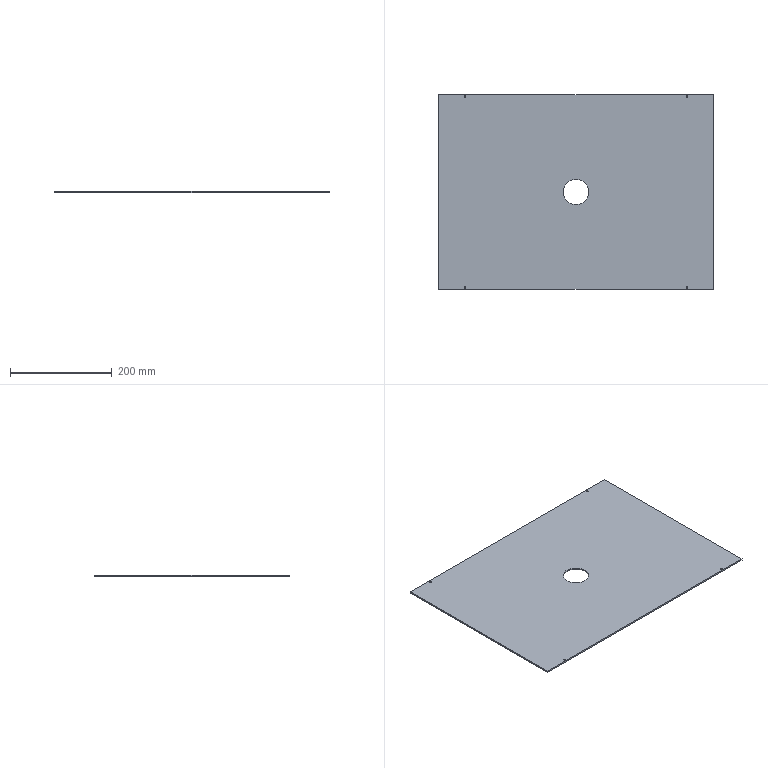Part | SolidWorks | features BaseBody 1 | 1 solid | 28 faces | box 540 x 382 x 3 mm | volume 612788 mm3 | cylinder 18 | plane 10 | commonest cylinder face diameters 3.3 x8 4.5 x8 50 x2
STEP:
#1=CARTESIAN_POINT('',(-25.,0.,0.));
#2=VERTEX_POINT('',#1);
#3=CARTESIAN_POINT('',(25.,0.,0.));
#4=VERTEX_POINT('',#3);
#5=CARTESIAN_POINT('',(0.,0.,0.));
#6=DIRECTION('',(0.,0.,1.));
#7=DIRECTION('',(1.,0.,0.));
#8=AXIS2_PLACEMENT_3D('',#5,#6,#7);
#9=CIRCLE('',#8,25.);
#10=EDGE_CURVE('',#2,#4,#9,.T.);
#11=ORIENTED_EDGE('',*,*,#10,.F.);
#12=CARTESIAN_POINT('',(-25.,0.,3.));
#13=VERTEX_POINT('',#12);
#14=CARTESIAN_POINT('',(-25.,0.,0.));
#15=DIRECTION('',(0.,0.,1.));
#16=VECTOR('',#15,1000.);
#17=LINE('',#14,#16);
#18=EDGE_CURVE('',#2,#13,#17,.T.);
#19=ORIENTED_EDGE('',*,*,#18,.T.);
#20=CARTESIAN_POINT('',(25.,0.,3.));
#21=VERTEX_POINT('',#20);
#22=CARTESIAN_POINT('',(0.,0.,3.));
#23=DIRECTION('',(0.,0.,-1.));
#24=DIRECTION('',(1.,0.,0.));
#25=AXIS2_PLACEMENT_3D('',#22,#23,#24);
#26=CIRCLE('',#25,25.);
#27=EDGE_CURVE('',#21,#13,#26,.T.);
#28=ORIENTED_EDGE('',*,*,#27,.F.);
#29=CARTESIAN_POINT('',(25.,0.,0.));
#30=DIRECTION('',(0.,0.,1.));
#31=VECTOR('',#30,1000.);
#32=LINE('',#29,#31);
#33=EDGE_CURVE('',#4,#21,#32,.T.);
#34=ORIENTED_EDGE('',*,*,#33,.F.);
#35=EDGE_LOOP('',(#11,#19,#28,#34));
#36=FACE_OUTER_BOUND('',#35,.T.);
#37=CARTESIAN_POINT('',(0.,0.,0.));
#38=DIRECTION('',(0.,0.,1.));
#39=DIRECTION('',(1.,0.,0.));
#40=AXIS2_PLACEMENT_3D('',#37,#38,#39);
#41=CYLINDRICAL_SURFACE('',#40,25.);
#42=ADVANCED_FACE('',(#36),#41,.F.);
#43=CARTESIAN_POINT('',(216.35,-187.,2.));
#44=VERTEX_POINT('',#43);
#45=CARTESIAN_POINT('',(219.65,-187.,2.));
#46=VERTEX_POINT('',#45);
#47=CARTESIAN_POINT('',(218.,-187.,2.));
#48=DIRECTION('',(0.,0.,1.));
#49=DIRECTION('',(1.,0.,0.));
#50=AXIS2_PLACEMENT_3D('',#47,#48,#49);
#51=CIRCLE('',#50,1.65);
#52=EDGE_CURVE('',#44,#46,#51,.T.);
#53=ORIENTED_EDGE('',*,*,#52,.F.);
#54=CARTESIAN_POINT('',(216.35,-187.,3.));
#55=VERTEX_POINT('',#54);
#56=CARTESIAN_POINT('',(216.35,-187.,5.));
#57=DIRECTION('',(0.,0.,1.));
#58=VECTOR('',#57,1000.);
#59=LINE('',#56,#58);
#60=EDGE_CURVE('',#44,#55,#59,.T.);
#61=ORIENTED_EDGE('',*,*,#60,.T.);
#62=CARTESIAN_POINT('',(219.65,-187.,3.));
#63=VERTEX_POINT('',#62);
#64=CARTESIAN_POINT('',(218.,-187.,3.));
#65=DIRECTION('',(0.,0.,-1.));
#66=DIRECTION('',(1.,0.,0.));
#67=AXIS2_PLACEMENT_3D('',#64,#65,#66);
#68=CIRCLE('',#67,1.65);
#69=EDGE_CURVE('',#63,#55,#68,.T.);
#70=ORIENTED_EDGE('',*,*,#69,.F.);
#71=CARTESIAN_POINT('',(219.65,-187.,5.));
#72=DIRECTION('',(0.,0.,1.));
#73=VECTOR('',#72,1000.);
#74=LINE('',#71,#73);
#75=EDGE_CURVE('',#46,#63,#74,.T.);
#76=ORIENTED_EDGE('',*,*,#75,.F.);
#77=EDGE_LOOP('',(#53,#61,#70,#76));
#78=FACE_OUTER_BOUND('',#77,.T.);
#79=CARTESIAN_POINT('',(218.,-187.,5.));
#80=DIRECTION('',(0.,0.,1.));
#81=DIRECTION('',(1.,0.,0.));
#82=AXIS2_PLACEMENT_3D('',#79,#80,#81);
#83=CYLINDRICAL_SURFACE('',#82,1.65);
#84=ADVANCED_FACE('',(#78),#83,.F.);
#85=CARTESIAN_POINT('',(-219.65,-187.,2.));
#86=VERTEX_POINT('',#85);
#87=CARTESIAN_POINT('',(-216.35,-187.,2.));
#88=VERTEX_POINT('',#87);
#89=CARTESIAN_POINT('',(-218.,-187.,2.));
#90=DIRECTION('',(0.,0.,1.));
#91=DIRECTION('',(1.,0.,0.));
#92=AXIS2_PLACEMENT_3D('',#89,#90,#91);
#93=CIRCLE('',#92,1.65);
#94=EDGE_CURVE('',#86,#88,#93,.T.);
#95=ORIENTED_EDGE('',*,*,#94,.F.);
#96=CARTESIAN_POINT('',(-219.65,-187.,3.));
#97=VERTEX_POINT('',#96);
#98=CARTESIAN_POINT('',(-219.65,-187.,5.));
#99=DIRECTION('',(0.,0.,1.));
#100=VECTOR('',#99,1000.);
#101=LINE('',#98,#100);
#102=EDGE_CURVE('',#86,#97,#101,.T.);
#103=ORIENTED_EDGE('',*,*,#102,.T.);
#104=CARTESIAN_POINT('',(-216.35,-187.,3.));
#105=VERTEX_POINT('',#104);
#106=CARTESIAN_POINT('',(-218.,-187.,3.));
#107=DIRECTION('',(0.,0.,-1.));
#108=DIRECTION('',(1.,0.,0.));
#109=AXIS2_PLACEMENT_3D('',#106,#107,#108);
#110=CIRCLE('',#109,1.65);
#111=EDGE_CURVE('',#105,#97,#110,.T.);
#112=ORIENTED_EDGE('',*,*,#111,.F.);
#113=CARTESIAN_POINT('',(-216.35,-187.,5.));
#114=DIRECTION('',(0.,0.,1.));
#115=VECTOR('',#114,1000.);
#116=LINE('',#113,#115);
#117=EDGE_CURVE('',#88,#105,#116,.T.);
#118=ORIENTED_EDGE('',*,*,#117,.F.);
#119=EDGE_LOOP('',(#95,#103,#112,#118));
#120=FACE_OUTER_BOUND('',#119,.T.);
#121=CARTESIAN_POINT('',(-218.,-187.,5.));
#122=DIRECTION('',(0.,0.,1.));
#123=DIRECTION('',(1.,0.,0.));
#124=AXIS2_PLACEMENT_3D('',#121,#122,#123);
#125=CYLINDRICAL_SURFACE('',#124,1.65);
#126=ADVANCED_FACE('',(#120),#125,.F.);
#127=CARTESIAN_POINT('',(219.65,187.,3.));
#128=VERTEX_POINT('',#127);
#129=CARTESIAN_POINT('',(216.35,187.,3.));
#130=VERTEX_POINT('',#129);
#131=CARTESIAN_POINT('',(218.,187.,3.));
#132=DIRECTION('',(0.,0.,-1.));
#133=DIRECTION('',(-1.,0.,0.));
#134=AXIS2_PLACEMENT_3D('',#131,#132,#133);
#135=CIRCLE('',#134,1.65);
#136=EDGE_CURVE('',#128,#130,#135,.T.);
#137=ORIENTED_EDGE('',*,*,#136,.F.);
#138=CARTESIAN_POINT('',(219.65,187.,2.));
#139=VERTEX_POINT('',#138);
#140=CARTESIAN_POINT('',(219.65,187.,5.));
#141=DIRECTION('',(0.,0.,-1.));
#142=VECTOR('',#141,1000.);
#143=LINE('',#140,#142);
#144=EDGE_CURVE('',#128,#139,#143,.T.);
#145=ORIENTED_EDGE('',*,*,#144,.T.);
#146=CARTESIAN_POINT('',(216.35,187.,2.));
#147=VERTEX_POINT('',#146);
#148=CARTESIAN_POINT('',(218.,187.,2.));
#149=DIRECTION('',(0.,0.,1.));
#150=DIRECTION('',(-1.,0.,0.));
#151=AXIS2_PLACEMENT_3D('',#148,#149,#150);
#152=CIRCLE('',#151,1.65);
#153=EDGE_CURVE('',#147,#139,#152,.T.);
#154=ORIENTED_EDGE('',*,*,#153,.F.);
#155=CARTESIAN_POINT('',(216.35,187.,5.));
#156=DIRECTION('',(0.,0.,-1.));
#157=VECTOR('',#156,1000.);
#158=LINE('',#155,#157);
#159=EDGE_CURVE('',#130,#147,#158,.T.);
#160=ORIENTED_EDGE('',*,*,#159,.F.);
#161=EDGE_LOOP('',(#137,#145,#154,#160));
#162=FACE_OUTER_BOUND('',#161,.T.);
#163=CARTESIAN_POINT('',(218.,187.,5.));
#164=DIRECTION('',(0.,0.,-1.));
#165=DIRECTION('',(-1.,0.,0.));
#166=AXIS2_PLACEMENT_3D('',#163,#164,#165);
#167=CYLINDRICAL_SURFACE('',#166,1.65);
#168=ADVANCED_FACE('',(#162),#167,.F.);
#169=CARTESIAN_POINT('',(-216.35,187.,3.));
#170=VERTEX_POINT('',#169);
#171=CARTESIAN_POINT('',(-219.65,187.,3.));
#172=VERTEX_POINT('',#171);
#173=CARTESIAN_POINT('',(-218.,187.,3.));
#174=DIRECTION('',(0.,0.,-1.));
#175=DIRECTION('',(-1.,0.,0.));
#176=AXIS2_PLACEMENT_3D('',#173,#174,#175);
#177=CIRCLE('',#176,1.65);
#178=EDGE_CURVE('',#170,#172,#177,.T.);
#179=ORIENTED_EDGE('',*,*,#178,.F.);
#180=CARTESIAN_POINT('',(-216.35,187.,2.));
#181=VERTEX_POINT('',#180);
#182=CARTESIAN_POINT('',(-216.35,187.,5.));
#183=DIRECTION('',(0.,0.,-1.));
#184=VECTOR('',#183,1000.);
#185=LINE('',#182,#184);
#186=EDGE_CURVE('',#170,#181,#185,.T.);
#187=ORIENTED_EDGE('',*,*,#186,.T.);
#188=CARTESIAN_POINT('',(-219.65,187.,2.));
#189=VERTEX_POINT('',#188);
#190=CARTESIAN_POINT('',(-218.,187.,2.));
#191=DIRECTION('',(0.,0.,1.));
#192=DIRECTION('',(-1.,0.,0.));
#193=AXIS2_PLACEMENT_3D('',#190,#191,#192);
#194=CIRCLE('',#193,1.65);
#195=EDGE_CURVE('',#189,#181,#194,.T.);
#196=ORIENTED_EDGE('',*,*,#195,.F.);
#197=CARTESIAN_POINT('',(-219.65,187.,5.));
#198=DIRECTION('',(0.,0.,-1.));
#199=VECTOR('',#198,1000.);
#200=LINE('',#197,#199);
#201=EDGE_CURVE('',#172,#189,#200,.T.);
#202=ORIENTED_EDGE('',*,*,#201,.F.);
#203=EDGE_LOOP('',(#179,#187,#196,#202));
#204=FACE_OUTER_BOUND('',#203,.T.);
#205=CARTESIAN_POINT('',(-218.,187.,5.));
#206=DIRECTION('',(0.,0.,-1.));
#207=DIRECTION('',(-1.,0.,0.));
#208=AXIS2_PLACEMENT_3D('',#205,#206,#207);
#209=CYLINDRICAL_SURFACE('',#208,1.65);
#210=ADVANCED_FACE('',(#204),#209,.F.);
#211=CARTESIAN_POINT('',(220.25,-187.,0.));
#212=VERTEX_POINT('',#211);
#213=CARTESIAN_POINT('',(215.75,-187.,0.));
#214=VERTEX_POINT('',#213);
#215=CARTESIAN_POINT('',(218.,-187.,0.));
#216=DIRECTION('',(0.,0.,-1.));
#217=DIRECTION('',(1.,0.,0.));
#218=AXIS2_PLACEMENT_3D('',#215,#216,#217);
#219=CIRCLE('',#218,2.25);
#220=EDGE_CURVE('',#212,#214,#219,.T.);
#221=ORIENTED_EDGE('',*,*,#220,.T.);
#222=CARTESIAN_POINT('',(215.75,-187.,2.));
#223=VERTEX_POINT('',#222);
#224=CARTESIAN_POINT('',(215.75,-187.,1.));
#225=DIRECTION('',(0.,0.,1.));
#226=VECTOR('',#225,1000.);
#227=LINE('',#224,#226);
#228=EDGE_CURVE('',#214,#223,#227,.T.);
#229=ORIENTED_EDGE('',*,*,#228,.T.);
#230=CARTESIAN_POINT('',(220.25,-187.,2.));
#231=VERTEX_POINT('',#230);
#232=CARTESIAN_POINT('',(218.,-187.,2.));
#233=DIRECTION('',(0.,0.,1.));
#234=DIRECTION('',(1.,0.,0.));
#235=AXIS2_PLACEMENT_3D('',#232,#233,#234);
#236=CIRCLE('',#235,2.25);
#237=EDGE_CURVE('',#223,#231,#236,.T.);
#238=ORIENTED_EDGE('',*,*,#237,.T.);
#239=CARTESIAN_POINT('',(220.25,-187.,1.));
#240=DIRECTION('',(0.,0.,1.));
#241=VECTOR('',#240,1000.);
#242=LINE('',#239,#241);
#243=EDGE_CURVE('',#212,#231,#242,.T.);
#244=ORIENTED_EDGE('',*,*,#243,.F.);
#245=EDGE_LOOP('',(#221,#229,#238,#244));
#246=FACE_OUTER_BOUND('',#245,.T.);
#247=CARTESIAN_POINT('',(218.,-187.,1.));
#248=DIRECTION('',(0.,0.,1.));
#249=DIRECTION('',(1.,0.,0.));
#250=AXIS2_PLACEMENT_3D('',#247,#248,#249);
#251=CYLINDRICAL_SURFACE('',#250,2.25);
#252=ADVANCED_FACE('',(#246),#251,.F.);
#253=CARTESIAN_POINT('',(-215.75,-187.,0.));
#254=VERTEX_POINT('',#253);
#255=CARTESIAN_POINT('',(-220.25,-187.,0.));
#256=VERTEX_POINT('',#255);
#257=CARTESIAN_POINT('',(-218.,-187.,0.));
#258=DIRECTION('',(0.,0.,-1.));
#259=DIRECTION('',(1.,0.,0.));
#260=AXIS2_PLACEMENT_3D('',#257,#258,#259);
#261=CIRCLE('',#260,2.25);
#262=EDGE_CURVE('',#254,#256,#261,.T.);
#263=ORIENTED_EDGE('',*,*,#262,.T.);
#264=CARTESIAN_POINT('',(-220.25,-187.,2.));
#265=VERTEX_POINT('',#264);
#266=CARTESIAN_POINT('',(-220.25,-187.,1.));
#267=DIRECTION('',(0.,0.,1.));
#268=VECTOR('',#267,1000.);
#269=LINE('',#266,#268);
#270=EDGE_CURVE('',#256,#265,#269,.T.);
#271=ORIENTED_EDGE('',*,*,#270,.T.);
#272=CARTESIAN_POINT('',(-215.75,-187.,2.));
#273=VERTEX_POINT('',#272);
#274=CARTESIAN_POINT('',(-218.,-187.,2.));
#275=DIRECTION('',(0.,0.,1.));
#276=DIRECTION('',(1.,0.,0.));
#277=AXIS2_PLACEMENT_3D('',#274,#275,#276);
#278=CIRCLE('',#277,2.25);
#279=EDGE_CURVE('',#265,#273,#278,.T.);
#280=ORIENTED_EDGE('',*,*,#279,.T.);
#281=CARTESIAN_POINT('',(-215.75,-187.,1.));
#282=DIRECTION('',(0.,0.,1.));
#283=VECTOR('',#282,1000.);
#284=LINE('',#281,#283);
#285=EDGE_CURVE('',#254,#273,#284,.T.);
#286=ORIENTED_EDGE('',*,*,#285,.F.);
#287=EDGE_LOOP('',(#263,#271,#280,#286));
#288=FACE_OUTER_BOUND('',#287,.T.);
#289=CARTESIAN_POINT('',(-218.,-187.,1.));
#290=DIRECTION('',(0.,0.,1.));
#291=DIRECTION('',(1.,0.,0.));
#292=AXIS2_PLACEMENT_3D('',#289,#290,#291);
#293=CYLINDRICAL_SURFACE('',#292,2.25);
#294=ADVANCED_FACE('',(#288),#293,.F.);
#295=CARTESIAN_POINT('',(220.25,187.,2.));
#296=VERTEX_POINT('',#295);
#297=CARTESIAN_POINT('',(215.75,187.,2.));
#298=VERTEX_POINT('',#297);
#299=CARTESIAN_POINT('',(218.,187.,2.));
#300=DIRECTION('',(0.,0.,-1.));
#301=DIRECTION('',(-1.,0.,0.));
#302=AXIS2_PLACEMENT_3D('',#299,#300,#301);
#303=CIRCLE('',#302,2.25);
#304=EDGE_CURVE('',#296,#298,#303,.T.);
#305=ORIENTED_EDGE('',*,*,#304,.F.);
#306=CARTESIAN_POINT('',(220.25,187.,0.));
#307=VERTEX_POINT('',#306);
#308=CARTESIAN_POINT('',(220.25,187.,1.));
#309=DIRECTION('',(0.,0.,-1.));
#310=VECTOR('',#309,1000.);
#311=LINE('',#308,#310);
#312=EDGE_CURVE('',#296,#307,#311,.T.);
#313=ORIENTED_EDGE('',*,*,#312,.T.);
#314=CARTESIAN_POINT('',(215.75,187.,0.));
#315=VERTEX_POINT('',#314);
#316=CARTESIAN_POINT('',(218.,187.,0.));
#317=DIRECTION('',(0.,0.,-1.));
#318=DIRECTION('',(-1.,0.,0.));
#319=AXIS2_PLACEMENT_3D('',#316,#317,#318);
#320=CIRCLE('',#319,2.25);
#321=EDGE_CURVE('',#307,#315,#320,.T.);
#322=ORIENTED_EDGE('',*,*,#321,.T.);
#323=CARTESIAN_POINT('',(215.75,187.,1.));
#324=DIRECTION('',(0.,0.,-1.));
#325=VECTOR('',#324,1000.);
#326=LINE('',#323,#325);
#327=EDGE_CURVE('',#298,#315,#326,.T.);
#328=ORIENTED_EDGE('',*,*,#327,.F.);
#329=EDGE_LOOP('',(#305,#313,#322,#328));
#330=FACE_OUTER_BOUND('',#329,.T.);
#331=CARTESIAN_POINT('',(218.,187.,1.));
#332=DIRECTION('',(0.,0.,-1.));
#333=DIRECTION('',(-1.,0.,0.));
#334=AXIS2_PLACEMENT_3D('',#331,#332,#333);
#335=CYLINDRICAL_SURFACE('',#334,2.25);
#336=ADVANCED_FACE('',(#330),#335,.F.);
#337=CARTESIAN_POINT('',(-215.75,187.,2.));
#338=VERTEX_POINT('',#337);
#339=CARTESIAN_POINT('',(-220.25,187.,2.));
#340=VERTEX_POINT('',#339);
#341=CARTESIAN_POINT('',(-218.,187.,2.));
#342=DIRECTION('',(0.,0.,-1.));
#343=DIRECTION('',(-1.,0.,0.));
#344=AXIS2_PLACEMENT_3D('',#341,#342,#343);
#345=CIRCLE('',#344,2.25);
#346=EDGE_CURVE('',#338,#340,#345,.T.);
#347=ORIENTED_EDGE('',*,*,#346,.F.);
#348=CARTESIAN_POINT('',(-215.75,187.,0.));
#349=VERTEX_POINT('',#348);
#350=CARTESIAN_POINT('',(-215.75,187.,1.));
#351=DIRECTION('',(0.,0.,-1.));
#352=VECTOR('',#351,1000.);
#353=LINE('',#350,#352);
#354=EDGE_CURVE('',#338,#349,#353,.T.);
#355=ORIENTED_EDGE('',*,*,#354,.T.);
#356=CARTESIAN_POINT('',(-220.25,187.,0.));
#357=VERTEX_POINT('',#356);
#358=CARTESIAN_POINT('',(-218.,187.,0.));
#359=DIRECTION('',(0.,0.,-1.));
#360=DIRECTION('',(-1.,0.,0.));
#361=AXIS2_PLACEMENT_3D('',#358,#359,#360);
#362=CIRCLE('',#361,2.25);
#363=EDGE_CURVE('',#349,#357,#362,.T.);
#364=ORIENTED_EDGE('',*,*,#363,.T.);
#365=CARTESIAN_POINT('',(-220.25,187.,1.));
#366=DIRECTION('',(0.,0.,-1.));
#367=VECTOR('',#366,1000.);
#368=LINE('',#365,#367);
#369=EDGE_CURVE('',#340,#357,#368,.T.);
#370=ORIENTED_EDGE('',*,*,#369,.F.);
#371=EDGE_LOOP('',(#347,#355,#364,#370));
#372=FACE_OUTER_BOUND('',#371,.T.);
#373=CARTESIAN_POINT('',(-218.,187.,1.));
#374=DIRECTION('',(0.,0.,-1.));
#375=DIRECTION('',(-1.,0.,0.));
#376=AXIS2_PLACEMENT_3D('',#373,#374,#375);
#377=CYLINDRICAL_SURFACE('',#376,2.25);
#378=ADVANCED_FACE('',(#372),#377,.F.);
#379=ORIENTED_EDGE('',*,*,#27,.T.);
#380=CARTESIAN_POINT('',(0.,0.,3.));
#381=DIRECTION('',(0.,0.,-1.));
#382=DIRECTION('',(1.,0.,0.));
#383=AXIS2_PLACEMENT_3D('',#380,#381,#382);
#384=CIRCLE('',#383,25.);
#385=EDGE_CURVE('',#13,#21,#384,.T.);
#386=ORIENTED_EDGE('',*,*,#385,.T.);
#387=EDGE_LOOP('',(#379,#386));
#388=FACE_BOUND('',#387,.T.);
#389=ORIENTED_EDGE('',*,*,#69,.T.);
#390=CARTESIAN_POINT('',(218.,-187.,3.));
#391=DIRECTION('',(0.,0.,-1.));
#392=DIRECTION('',(1.,0.,0.));
#393=AXIS2_PLACEMENT_3D('',#390,#391,#392);
#394=CIRCLE('',#393,1.65);
#395=EDGE_CURVE('',#55,#63,#394,.T.);
#396=ORIENTED_EDGE('',*,*,#395,.T.);
#397=EDGE_LOOP('',(#389,#396));
#398=FACE_BOUND('',#397,.T.);
#399=ORIENTED_EDGE('',*,*,#111,.T.);
#400=CARTESIAN_POINT('',(-218.,-187.,3.));
#401=DIRECTION('',(0.,0.,-1.));
#402=DIRECTION('',(1.,0.,0.));
#403=AXIS2_PLACEMENT_3D('',#400,#401,#402);
#404=CIRCLE('',#403,1.65);
#405=EDGE_CURVE('',#97,#105,#404,.T.);
#406=ORIENTED_EDGE('',*,*,#405,.T.);
#407=EDGE_LOOP('',(#399,#406));
#408=FACE_BOUND('',#407,.T.);
#409=CARTESIAN_POINT('',(218.,187.,3.));
#410=DIRECTION('',(0.,0.,-1.));
#411=DIRECTION('',(-1.,0.,0.));
#412=AXIS2_PLACEMENT_3D('',#409,#410,#411);
#413=CIRCLE('',#412,1.65);
#414=EDGE_CURVE('',#130,#128,#413,.T.);
#415=ORIENTED_EDGE('',*,*,#414,.T.);
#416=ORIENTED_EDGE('',*,*,#136,.T.);
#417=EDGE_LOOP('',(#415,#416));
#418=FACE_BOUND('',#417,.T.);
#419=CARTESIAN_POINT('',(-218.,187.,3.));
#420=DIRECTION('',(0.,0.,-1.));
#421=DIRECTION('',(-1.,0.,0.));
#422=AXIS2_PLACEMENT_3D('',#419,#420,#421);
#423=CIRCLE('',#422,1.65);
#424=EDGE_CURVE('',#172,#170,#423,.T.);
#425=ORIENTED_EDGE('',*,*,#424,.T.);
#426=ORIENTED_EDGE('',*,*,#178,.T.);
#427=EDGE_LOOP('',(#425,#426));
#428=FACE_BOUND('',#427,.T.);
#429=CARTESIAN_POINT('',(-270.,-191.,3.));
#430=VERTEX_POINT('',#429);
#431=CARTESIAN_POINT('',(270.,-191.,3.));
#432=VERTEX_POINT('',#431);
#433=CARTESIAN_POINT('',(0.,-191.,3.));
#434=DIRECTION('',(1.,0.,0.));
#435=VECTOR('',#434,1000.);
#436=LINE('',#433,#435);
#437=EDGE_CURVE('',#430,#432,#436,.T.);
#438=ORIENTED_EDGE('',*,*,#437,.T.);
#439=CARTESIAN_POINT('',(270.,191.,3.));
#440=VERTEX_POINT('',#439);
#441=CARTESIAN_POINT('',(270.,0.,3.));
#442=DIRECTION('',(0.,1.,0.));
#443=VECTOR('',#442,1000.);
#444=LINE('',#441,#443);
#445=EDGE_CURVE('',#432,#440,#444,.T.);
#446=ORIENTED_EDGE('',*,*,#445,.T.);
#447=CARTESIAN_POINT('',(-270.,191.,3.));
#448=VERTEX_POINT('',#447);
#449=CARTESIAN_POINT('',(0.,191.,3.));
#450=DIRECTION('',(-1.,0.,0.));
#451=VECTOR('',#450,1000.);
#452=LINE('',#449,#451);
#453=EDGE_CURVE('',#440,#448,#452,.T.);
#454=ORIENTED_EDGE('',*,*,#453,.T.);
#455=CARTESIAN_POINT('',(-270.,0.,3.));
#456=DIRECTION('',(0.,-1.,0.));
#457=VECTOR('',#456,1000.);
#458=LINE('',#455,#457);
#459=EDGE_CURVE('',#448,#430,#458,.T.);
#460=ORIENTED_EDGE('',*,*,#459,.T.);
#461=EDGE_LOOP('',(#438,#446,#454,#460));
#462=FACE_OUTER_BOUND('',#461,.T.);
#463=CARTESIAN_POINT('',(0.,0.,3.));
#464=DIRECTION('',(0.,0.,1.));
#465=DIRECTION('',(1.,0.,0.));
#466=AXIS2_PLACEMENT_3D('',#463,#464,#465);
#467=PLANE('',#466);
#468=ADVANCED_FACE('',(#388,#398,#408,#418,#428,#462),#467,.T.);
#469=ORIENTED_EDGE('',*,*,#18,.F.);
#470=CARTESIAN_POINT('',(0.,0.,0.));
#471=DIRECTION('',(0.,0.,1.));
#472=DIRECTION('',(1.,0.,0.));
#473=AXIS2_PLACEMENT_3D('',#470,#471,#472);
#474=CIRCLE('',#473,25.);
#475=EDGE_CURVE('',#4,#2,#474,.T.);
#476=ORIENTED_EDGE('',*,*,#475,.F.);
#477=ORIENTED_EDGE('',*,*,#33,.T.);
#478=ORIENTED_EDGE('',*,*,#385,.F.);
#479=EDGE_LOOP('',(#469,#476,#477,#478));
#480=FACE_OUTER_BOUND('',#479,.T.);
#481=CARTESIAN_POINT('',(0.,0.,0.));
#482=DIRECTION('',(0.,0.,1.));
#483=DIRECTION('',(1.,0.,0.));
#484=AXIS2_PLACEMENT_3D('',#481,#482,#483);
#485=CYLINDRICAL_SURFACE('',#484,25.);
#486=ADVANCED_FACE('',(#480),#485,.F.);
#487=ORIENTED_EDGE('',*,*,#60,.F.);
#488=CARTESIAN_POINT('',(218.,-187.,2.));
#489=DIRECTION('',(0.,0.,1.));
#490=DIRECTION('',(1.,0.,0.));
#491=AXIS2_PLACEMENT_3D('',#488,#489,#490);
#492=CIRCLE('',#491,1.65);
#493=EDGE_CURVE('',#46,#44,#492,.T.);
#494=ORIENTED_EDGE('',*,*,#493,.F.);
#495=ORIENTED_EDGE('',*,*,#75,.T.);
#496=ORIENTED_EDGE('',*,*,#395,.F.);
#497=EDGE_LOOP('',(#487,#494,#495,#496));
#498=FACE_OUTER_BOUND('',#497,.T.);
#499=CARTESIAN_POINT('',(218.,-187.,5.));
#500=DIRECTION('',(0.,0.,1.));
#501=DIRECTION('',(1.,0.,0.));
#502=AXIS2_PLACEMENT_3D('',#499,#500,#501);
#503=CYLINDRICAL_SURFACE('',#502,1.65);
#504=ADVANCED_FACE('',(#498),#503,.F.);
#505=ORIENTED_EDGE('',*,*,#102,.F.);
#506=CARTESIAN_POINT('',(-218.,-187.,2.));
#507=DIRECTION('',(0.,0.,1.));
#508=DIRECTION('',(1.,0.,0.));
#509=AXIS2_PLACEMENT_3D('',#506,#507,#508);
#510=CIRCLE('',#509,1.65);
#511=EDGE_CURVE('',#88,#86,#510,.T.);
#512=ORIENTED_EDGE('',*,*,#511,.F.);
#513=ORIENTED_EDGE('',*,*,#117,.T.);
#514=ORIENTED_EDGE('',*,*,#405,.F.);
#515=EDGE_LOOP('',(#505,#512,#513,#514));
#516=FACE_OUTER_BOUND('',#515,.T.);
#517=CARTESIAN_POINT('',(-218.,-187.,5.));
#518=DIRECTION('',(0.,0.,1.));
#519=DIRECTION('',(1.,0.,0.));
#520=AXIS2_PLACEMENT_3D('',#517,#518,#519);
#521=CYLINDRICAL_SURFACE('',#520,1.65);
#522=ADVANCED_FACE('',(#516),#521,.F.);
#523=ORIENTED_EDGE('',*,*,#144,.F.);
#524=ORIENTED_EDGE('',*,*,#414,.F.);
#525=ORIENTED_EDGE('',*,*,#159,.T.);
#526=CARTESIAN_POINT('',(218.,187.,2.));
#527=DIRECTION('',(0.,0.,1.));
#528=DIRECTION('',(-1.,0.,0.));
#529=AXIS2_PLACEMENT_3D('',#526,#527,#528);
#530=CIRCLE('',#529,1.65);
#531=EDGE_CURVE('',#139,#147,#530,.T.);
#532=ORIENTED_EDGE('',*,*,#531,.F.);
#533=EDGE_LOOP('',(#523,#524,#525,#532));
#534=FACE_OUTER_BOUND('',#533,.T.);
#535=CARTESIAN_POINT('',(218.,187.,5.));
#536=DIRECTION('',(0.,0.,-1.));
#537=DIRECTION('',(-1.,0.,0.));
#538=AXIS2_PLACEMENT_3D('',#535,#536,#537);
#539=CYLINDRICAL_SURFACE('',#538,1.65);
#540=ADVANCED_FACE('',(#534),#539,.F.);
#541=ORIENTED_EDGE('',*,*,#186,.F.);
#542=ORIENTED_EDGE('',*,*,#424,.F.);
#543=ORIENTED_EDGE('',*,*,#201,.T.);
#544=CARTESIAN_POINT('',(-218.,187.,2.));
#545=DIRECTION('',(0.,0.,1.));
#546=DIRECTION('',(-1.,0.,0.));
#547=AXIS2_PLACEMENT_3D('',#544,#545,#546);
#548=CIRCLE('',#547,1.65);
#549=EDGE_CURVE('',#181,#189,#548,.T.);
#550=ORIENTED_EDGE('',*,*,#549,.F.);
#551=EDGE_LOOP('',(#541,#542,#543,#550));
#552=FACE_OUTER_BOUND('',#551,.T.);
#553=CARTESIAN_POINT('',(-218.,187.,5.));
#554=DIRECTION('',(0.,0.,-1.));
#555=DIRECTION('',(-1.,0.,0.));
#556=AXIS2_PLACEMENT_3D('',#553,#554,#555);
#557=CYLINDRICAL_SURFACE('',#556,1.65);
#558=ADVANCED_FACE('',(#552),#557,.F.);
#559=ORIENTED_EDGE('',*,*,#445,.F.);
#560=CARTESIAN_POINT('',(270.,-191.,0.));
#561=VERTEX_POINT('',#560);
#562=CARTESIAN_POINT('',(270.,-191.,0.));
#563=DIRECTION('',(0.,0.,-1.));
#564=VECTOR('',#563,1000.);
#565=LINE('',#562,#564);
#566=EDGE_CURVE('',#432,#561,#565,.T.);
#567=ORIENTED_EDGE('',*,*,#566,.T.);
#568=CARTESIAN_POINT('',(270.,191.,0.));
#569=VERTEX_POINT('',#568);
#570=CARTESIAN_POINT('',(270.,-191.,0.));
#571=DIRECTION('',(0.,1.,0.));
#572=VECTOR('',#571,1000.);
#573=LINE('',#570,#572);
#574=EDGE_CURVE('',#561,#569,#573,.T.);
#575=ORIENTED_EDGE('',*,*,#574,.T.);
#576=CARTESIAN_POINT('',(270.,191.,0.));
#577=DIRECTION('',(0.,0.,1.));
#578=VECTOR('',#577,1000.);
#579=LINE('',#576,#578);
#580=EDGE_CURVE('',#569,#440,#579,.T.);
#581=ORIENTED_EDGE('',*,*,#580,.T.);
#582=EDGE_LOOP('',(#559,#567,#575,#581));
#583=FACE_OUTER_BOUND('',#582,.T.);
#584=CARTESIAN_POINT('',(270.,-191.,0.));
#585=DIRECTION('',(1.,0.,0.));
#586=DIRECTION('',(0.,1.,0.));
#587=AXIS2_PLACEMENT_3D('',#584,#585,#586);
#588=PLANE('',#587);
#589=ADVANCED_FACE('',(#583),#588,.T.);
#590=ORIENTED_EDGE('',*,*,#437,.F.);
#591=CARTESIAN_POINT('',(-270.,-191.,0.));
#592=VERTEX_POINT('',#591);
#593=CARTESIAN_POINT('',(-270.,-191.,0.));
#594=DIRECTION('',(0.,0.,-1.));
#595=VECTOR('',#594,1000.);
#596=LINE('',#593,#595);
#597=EDGE_CURVE('',#430,#592,#596,.T.);
#598=ORIENTED_EDGE('',*,*,#597,.T.);
#599=CARTESIAN_POINT('',(-270.,-191.,0.));
#600=DIRECTION('',(1.,0.,0.));
#601=VECTOR('',#600,1000.);
#602=LINE('',#599,#601);
#603=EDGE_CURVE('',#592,#561,#602,.T.);
#604=ORIENTED_EDGE('',*,*,#603,.T.);
#605=ORIENTED_EDGE('',*,*,#566,.F.);
#606=EDGE_LOOP('',(#590,#598,#604,#605));
#607=FACE_OUTER_BOUND('',#606,.T.);
#608=CARTESIAN_POINT('',(-270.,-191.,0.));
#609=DIRECTION('',(0.,-1.,0.));
#610=DIRECTION('',(0.,0.,-1.));
#611=AXIS2_PLACEMENT_3D('',#608,#609,#610);
#612=PLANE('',#611);
#613=ADVANCED_FACE('',(#607),#612,.T.);
#614=ORIENTED_EDGE('',*,*,#459,.F.);
#615=CARTESIAN_POINT('',(-270.,191.,0.));
#616=VERTEX_POINT('',#615);
#617=CARTESIAN_POINT('',(-270.,191.,0.));
#618=DIRECTION('',(0.,0.,-1.));
#619=VECTOR('',#618,1000.);
#620=LINE('',#617,#619);
#621=EDGE_CURVE('',#448,#616,#620,.T.);
#622=ORIENTED_EDGE('',*,*,#621,.T.);
#623=CARTESIAN_POINT('',(-270.,191.,0.));
#624=DIRECTION('',(0.,-1.,0.));
#625=VECTOR('',#624,1000.);
#626=LINE('',#623,#625);
#627=EDGE_CURVE('',#616,#592,#626,.T.);
#628=ORIENTED_EDGE('',*,*,#627,.T.);
#629=ORIENTED_EDGE('',*,*,#597,.F.);
#630=EDGE_LOOP('',(#614,#622,#628,#629));
#631=FACE_OUTER_BOUND('',#630,.T.);
#632=CARTESIAN_POINT('',(-270.,191.,0.));
#633=DIRECTION('',(-1.,0.,0.));
#634=DIRECTION('',(0.,-1.,0.));
#635=AXIS2_PLACEMENT_3D('',#632,#633,#634);
#636=PLANE('',#635);
#637=ADVANCED_FACE('',(#631),#636,.T.);
#638=ORIENTED_EDGE('',*,*,#453,.F.);
#639=ORIENTED_EDGE('',*,*,#580,.F.);
#640=CARTESIAN_POINT('',(270.,191.,0.));
#641=DIRECTION('',(-1.,0.,0.));
#642=VECTOR('',#641,1000.);
#643=LINE('',#640,#642);
#644=EDGE_CURVE('',#569,#616,#643,.T.);
#645=ORIENTED_EDGE('',*,*,#644,.T.);
#646=ORIENTED_EDGE('',*,*,#621,.F.);
#647=EDGE_LOOP('',(#638,#639,#645,#646));
#648=FACE_OUTER_BOUND('',#647,.T.);
#649=CARTESIAN_POINT('',(270.,191.,0.));
#650=DIRECTION('',(0.,1.,0.));
#651=DIRECTION('',(-1.,0.,0.));
#652=AXIS2_PLACEMENT_3D('',#649,#650,#651);
#653=PLANE('',#652);
#654=ADVANCED_FACE('',(#648),#653,.T.);
#655=ORIENTED_EDGE('',*,*,#475,.T.);
#656=ORIENTED_EDGE('',*,*,#10,.T.);
#657=EDGE_LOOP('',(#655,#656));
#658=FACE_BOUND('',#657,.T.);
#659=ORIENTED_EDGE('',*,*,#220,.F.);
#660=CARTESIAN_POINT('',(218.,-187.,0.));
#661=DIRECTION('',(0.,0.,-1.));
#662=DIRECTION('',(1.,0.,0.));
#663=AXIS2_PLACEMENT_3D('',#660,#661,#662);
#664=CIRCLE('',#663,2.25);
#665=EDGE_CURVE('',#214,#212,#664,.T.);
#666=ORIENTED_EDGE('',*,*,#665,.F.);
#667=EDGE_LOOP('',(#659,#666));
#668=FACE_BOUND('',#667,.T.);
#669=ORIENTED_EDGE('',*,*,#262,.F.);
#670=CARTESIAN_POINT('',(-218.,-187.,0.));
#671=DIRECTION('',(0.,0.,-1.));
#672=DIRECTION('',(1.,0.,0.));
#673=AXIS2_PLACEMENT_3D('',#670,#671,#672);
#674=CIRCLE('',#673,2.25);
#675=EDGE_CURVE('',#256,#254,#674,.T.);
#676=ORIENTED_EDGE('',*,*,#675,.F.);
#677=EDGE_LOOP('',(#669,#676));
#678=FACE_BOUND('',#677,.T.);
#679=CARTESIAN_POINT('',(218.,187.,0.));
#680=DIRECTION('',(0.,0.,-1.));
#681=DIRECTION('',(-1.,0.,0.));
#682=AXIS2_PLACEMENT_3D('',#679,#680,#681);
#683=CIRCLE('',#682,2.25);
#684=EDGE_CURVE('',#315,#307,#683,.T.);
#685=ORIENTED_EDGE('',*,*,#684,.F.);
#686=ORIENTED_EDGE('',*,*,#321,.F.);
#687=EDGE_LOOP('',(#685,#686));
#688=FACE_BOUND('',#687,.T.);
#689=CARTESIAN_POINT('',(-218.,187.,0.));
#690=DIRECTION('',(0.,0.,-1.));
#691=DIRECTION('',(-1.,0.,0.));
#692=AXIS2_PLACEMENT_3D('',#689,#690,#691);
#693=CIRCLE('',#692,2.25);
#694=EDGE_CURVE('',#357,#349,#693,.T.);
#695=ORIENTED_EDGE('',*,*,#694,.F.);
#696=ORIENTED_EDGE('',*,*,#363,.F.);
#697=EDGE_LOOP('',(#695,#696));
#698=FACE_BOUND('',#697,.T.);
#699=ORIENTED_EDGE('',*,*,#574,.F.);
#700=ORIENTED_EDGE('',*,*,#603,.F.);
#701=ORIENTED_EDGE('',*,*,#627,.F.);
#702=ORIENTED_EDGE('',*,*,#644,.F.);
#703=EDGE_LOOP('',(#699,#700,#701,#702));
#704=FACE_OUTER_BOUND('',#703,.T.);
#705=CARTESIAN_POINT('',(0.,0.,0.));
#706=DIRECTION('',(0.,0.,1.));
#707=DIRECTION('',(1.,0.,0.));
#708=AXIS2_PLACEMENT_3D('',#705,#706,#707);
#709=PLANE('',#708);
#710=ADVANCED_FACE('',(#658,#668,#678,#688,#698,#704),#709,.F.);
#711=ORIENTED_EDGE('',*,*,#493,.T.);
#712=ORIENTED_EDGE('',*,*,#52,.T.);
#713=EDGE_LOOP('',(#711,#712));
#714=FACE_BOUND('',#713,.T.);
#715=CARTESIAN_POINT('',(218.,-187.,2.));
#716=DIRECTION('',(0.,0.,1.));
#717=DIRECTION('',(1.,0.,0.));
#718=AXIS2_PLACEMENT_3D('',#715,#716,#717);
#719=CIRCLE('',#718,2.25);
#720=EDGE_CURVE('',#231,#223,#719,.T.);
#721=ORIENTED_EDGE('',*,*,#720,.F.);
#722=ORIENTED_EDGE('',*,*,#237,.F.);
#723=EDGE_LOOP('',(#721,#722));
#724=FACE_OUTER_BOUND('',#723,.T.);
#725=CARTESIAN_POINT('',(218.,-187.,2.));
#726=DIRECTION('',(0.,0.,1.));
#727=DIRECTION('',(1.,0.,0.));
#728=AXIS2_PLACEMENT_3D('',#725,#726,#727);
#729=PLANE('',#728);
#730=ADVANCED_FACE('',(#714,#724),#729,.F.);
#731=ORIENTED_EDGE('',*,*,#511,.T.);
#732=ORIENTED_EDGE('',*,*,#94,.T.);
#733=EDGE_LOOP('',(#731,#732));
#734=FACE_BOUND('',#733,.T.);
#735=CARTESIAN_POINT('',(-218.,-187.,2.));
#736=DIRECTION('',(0.,0.,1.));
#737=DIRECTION('',(1.,0.,0.));
#738=AXIS2_PLACEMENT_3D('',#735,#736,#737);
#739=CIRCLE('',#738,2.25);
#740=EDGE_CURVE('',#273,#265,#739,.T.);
#741=ORIENTED_EDGE('',*,*,#740,.F.);
#742=ORIENTED_EDGE('',*,*,#279,.F.);
#743=EDGE_LOOP('',(#741,#742));
#744=FACE_OUTER_BOUND('',#743,.T.);
#745=CARTESIAN_POINT('',(-218.,-187.,2.));
#746=DIRECTION('',(0.,0.,1.));
#747=DIRECTION('',(1.,0.,0.));
#748=AXIS2_PLACEMENT_3D('',#745,#746,#747);
#749=PLANE('',#748);
#750=ADVANCED_FACE('',(#734,#744),#749,.F.);
#751=ORIENTED_EDGE('',*,*,#153,.T.);
#752=ORIENTED_EDGE('',*,*,#531,.T.);
#753=EDGE_LOOP('',(#751,#752));
#754=FACE_BOUND('',#753,.T.);
#755=CARTESIAN_POINT('',(218.,187.,2.));
#756=DIRECTION('',(0.,0.,-1.));
#757=DIRECTION('',(-1.,0.,0.));
#758=AXIS2_PLACEMENT_3D('',#755,#756,#757);
#759=CIRCLE('',#758,2.25);
#760=EDGE_CURVE('',#298,#296,#759,.T.);
#761=ORIENTED_EDGE('',*,*,#760,.T.);
#762=ORIENTED_EDGE('',*,*,#304,.T.);
#763=EDGE_LOOP('',(#761,#762));
#764=FACE_OUTER_BOUND('',#763,.T.);
#765=CARTESIAN_POINT('',(218.,187.,2.));
#766=DIRECTION('',(0.,0.,-1.));
#767=DIRECTION('',(-1.,0.,0.));
#768=AXIS2_PLACEMENT_3D('',#765,#766,#767);
#769=PLANE('',#768);
#770=ADVANCED_FACE('',(#754,#764),#769,.T.);
#771=ORIENTED_EDGE('',*,*,#195,.T.);
#772=ORIENTED_EDGE('',*,*,#549,.T.);
#773=EDGE_LOOP('',(#771,#772));
#774=FACE_BOUND('',#773,.T.);
#775=CARTESIAN_POINT('',(-218.,187.,2.));
#776=DIRECTION('',(0.,0.,-1.));
#777=DIRECTION('',(-1.,0.,0.));
#778=AXIS2_PLACEMENT_3D('',#775,#776,#777);
#779=CIRCLE('',#778,2.25);
#780=EDGE_CURVE('',#340,#338,#779,.T.);
#781=ORIENTED_EDGE('',*,*,#780,.T.);
#782=ORIENTED_EDGE('',*,*,#346,.T.);
#783=EDGE_LOOP('',(#781,#782));
#784=FACE_OUTER_BOUND('',#783,.T.);
#785=CARTESIAN_POINT('',(-218.,187.,2.));
#786=DIRECTION('',(0.,0.,-1.));
#787=DIRECTION('',(-1.,0.,0.));
#788=AXIS2_PLACEMENT_3D('',#785,#786,#787);
#789=PLANE('',#788);
#790=ADVANCED_FACE('',(#774,#784),#789,.T.);
#791=ORIENTED_EDGE('',*,*,#228,.F.);
#792=ORIENTED_EDGE('',*,*,#665,.T.);
#793=ORIENTED_EDGE('',*,*,#243,.T.);
#794=ORIENTED_EDGE('',*,*,#720,.T.);
#795=EDGE_LOOP('',(#791,#792,#793,#794));
#796=FACE_OUTER_BOUND('',#795,.T.);
#797=CARTESIAN_POINT('',(218.,-187.,1.));
#798=DIRECTION('',(0.,0.,1.));
#799=DIRECTION('',(1.,0.,0.));
#800=AXIS2_PLACEMENT_3D('',#797,#798,#799);
#801=CYLINDRICAL_SURFACE('',#800,2.25);
#802=ADVANCED_FACE('',(#796),#801,.F.);
#803=ORIENTED_EDGE('',*,*,#270,.F.);
#804=ORIENTED_EDGE('',*,*,#675,.T.);
#805=ORIENTED_EDGE('',*,*,#285,.T.);
#806=ORIENTED_EDGE('',*,*,#740,.T.);
#807=EDGE_LOOP('',(#803,#804,#805,#806));
#808=FACE_OUTER_BOUND('',#807,.T.);
#809=CARTESIAN_POINT('',(-218.,-187.,1.));
#810=DIRECTION('',(0.,0.,1.));
#811=DIRECTION('',(1.,0.,0.));
#812=AXIS2_PLACEMENT_3D('',#809,#810,#811);
#813=CYLINDRICAL_SURFACE('',#812,2.25);
#814=ADVANCED_FACE('',(#808),#813,.F.);
#815=ORIENTED_EDGE('',*,*,#312,.F.);
#816=ORIENTED_EDGE('',*,*,#760,.F.);
#817=ORIENTED_EDGE('',*,*,#327,.T.);
#818=ORIENTED_EDGE('',*,*,#684,.T.);
#819=EDGE_LOOP('',(#815,#816,#817,#818));
#820=FACE_OUTER_BOUND('',#819,.T.);
#821=CARTESIAN_POINT('',(218.,187.,1.));
#822=DIRECTION('',(0.,0.,-1.));
#823=DIRECTION('',(-1.,0.,0.));
#824=AXIS2_PLACEMENT_3D('',#821,#822,#823);
#825=CYLINDRICAL_SURFACE('',#824,2.25);
#826=ADVANCED_FACE('',(#820),#825,.F.);
#827=ORIENTED_EDGE('',*,*,#354,.F.);
#828=ORIENTED_EDGE('',*,*,#780,.F.);
#829=ORIENTED_EDGE('',*,*,#369,.T.);
#830=ORIENTED_EDGE('',*,*,#694,.T.);
#831=EDGE_LOOP('',(#827,#828,#829,#830));
#832=FACE_OUTER_BOUND('',#831,.T.);
#833=CARTESIAN_POINT('',(-218.,187.,1.));
#834=DIRECTION('',(0.,0.,-1.));
#835=DIRECTION('',(-1.,0.,0.));
#836=AXIS2_PLACEMENT_3D('',#833,#834,#835);
#837=CYLINDRICAL_SURFACE('',#836,2.25);
#838=ADVANCED_FACE('',(#832),#837,.F.);
#839=CLOSED_SHELL('',(#42,#84,#126,#168,#210,#252,#294,#336,#378,#468,#486,#504,#522,#540,#558,#589,#613,#637,#654,#710,#730,#750,#770,#790,#802,#814,#826,#838));
#840=MANIFOLD_SOLID_BREP('',#839);
#841=CARTESIAN_POINT('',(0.,0.,0.));
#842=DIRECTION('',(0.,0.,1.));
#843=DIRECTION('',(1.,0.,0.));
#844=AXIS2_PLACEMENT_3D('',#841,#842,#843);
#845=(LENGTH_UNIT()NAMED_UNIT(*)SI_UNIT(.MILLI.,.METRE.));
#846=UNCERTAINTY_MEASURE_WITH_UNIT(LENGTH_MEASURE(0.00001),#845,'','');
#847=(NAMED_UNIT(*)PLANE_ANGLE_UNIT()SI_UNIT($,.RADIAN.));
#848=(NAMED_UNIT(*)SI_UNIT($,.STERADIAN.)SOLID_ANGLE_UNIT());
#849=(GEOMETRIC_REPRESENTATION_CONTEXT(3)GLOBAL_UNCERTAINTY_ASSIGNED_CONTEXT((#846))GLOBAL_UNIT_ASSIGNED_CONTEXT((#845,#847,#848))REPRESENTATION_CONTEXT('',''));
#850=ADVANCED_BREP_SHAPE_REPRESENTATION('',(#840,#844),#849);